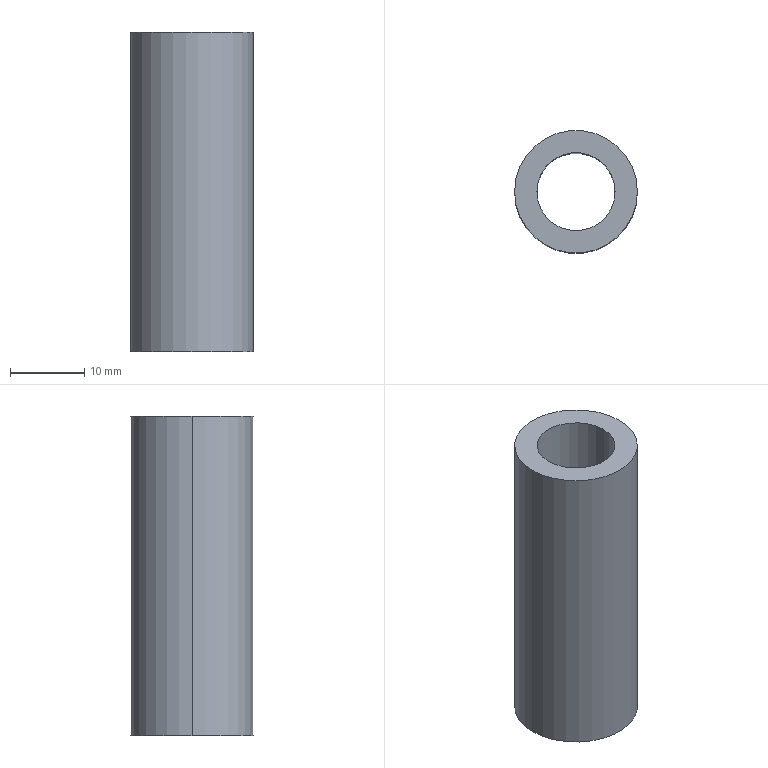Part | SolidWorks | features Extrusion 1, ICE 1 | 1 solid | 6 faces | box 16.5 x 16.5 x 43 mm | volume 5471 mm3 | cylinder 4 | plane 2 | commonest cylinder face diameters 10.5 x2 16.5 x2
STEP:
#1=CARTESIAN_POINT('',(-5.25,0.,0.));
#2=VERTEX_POINT('',#1);
#3=CARTESIAN_POINT('',(5.25,0.,0.));
#4=VERTEX_POINT('',#3);
#5=CARTESIAN_POINT('',(0.,0.,0.));
#6=DIRECTION('',(0.,0.,1.));
#7=DIRECTION('',(1.,0.,0.));
#8=AXIS2_PLACEMENT_3D('',#5,#6,#7);
#9=CIRCLE('',#8,5.25);
#10=EDGE_CURVE('',#2,#4,#9,.T.);
#11=ORIENTED_EDGE('',*,*,#10,.F.);
#12=CARTESIAN_POINT('',(-5.25,0.,43.));
#13=VERTEX_POINT('',#12);
#14=CARTESIAN_POINT('',(-5.25,0.,-57.));
#15=DIRECTION('',(0.,0.,1.));
#16=VECTOR('',#15,1000.);
#17=LINE('',#14,#16);
#18=EDGE_CURVE('',#2,#13,#17,.T.);
#19=ORIENTED_EDGE('',*,*,#18,.T.);
#20=CARTESIAN_POINT('',(5.25,0.,43.));
#21=VERTEX_POINT('',#20);
#22=CARTESIAN_POINT('',(0.,0.,43.));
#23=DIRECTION('',(0.,0.,1.));
#24=DIRECTION('',(1.,0.,0.));
#25=AXIS2_PLACEMENT_3D('',#22,#23,#24);
#26=CIRCLE('',#25,5.25);
#27=EDGE_CURVE('',#13,#21,#26,.T.);
#28=ORIENTED_EDGE('',*,*,#27,.T.);
#29=CARTESIAN_POINT('',(5.25,0.,-57.));
#30=DIRECTION('',(0.,0.,1.));
#31=VECTOR('',#30,1000.);
#32=LINE('',#29,#31);
#33=EDGE_CURVE('',#4,#21,#32,.T.);
#34=ORIENTED_EDGE('',*,*,#33,.F.);
#35=EDGE_LOOP('',(#11,#19,#28,#34));
#36=FACE_OUTER_BOUND('',#35,.T.);
#37=CARTESIAN_POINT('',(0.,0.,-57.));
#38=DIRECTION('',(0.,0.,1.));
#39=DIRECTION('',(1.,0.,0.));
#40=AXIS2_PLACEMENT_3D('',#37,#38,#39);
#41=CYLINDRICAL_SURFACE('',#40,5.25);
#42=ADVANCED_FACE('',(#36),#41,.F.);
#43=CARTESIAN_POINT('',(8.25,0.,43.));
#44=VERTEX_POINT('',#43);
#45=CARTESIAN_POINT('',(-8.25,0.,43.));
#46=VERTEX_POINT('',#45);
#47=CARTESIAN_POINT('',(0.,0.,43.));
#48=DIRECTION('',(0.,0.,1.));
#49=DIRECTION('',(1.,0.,0.));
#50=AXIS2_PLACEMENT_3D('',#47,#48,#49);
#51=CIRCLE('',#50,8.25);
#52=EDGE_CURVE('',#44,#46,#51,.T.);
#53=ORIENTED_EDGE('',*,*,#52,.F.);
#54=CARTESIAN_POINT('',(8.25,0.,0.));
#55=VERTEX_POINT('',#54);
#56=CARTESIAN_POINT('',(8.25,0.,43.));
#57=DIRECTION('',(0.,0.,-1.));
#58=VECTOR('',#57,1000.);
#59=LINE('',#56,#58);
#60=EDGE_CURVE('',#44,#55,#59,.T.);
#61=ORIENTED_EDGE('',*,*,#60,.T.);
#62=CARTESIAN_POINT('',(-8.25,0.,0.));
#63=VERTEX_POINT('',#62);
#64=CARTESIAN_POINT('',(0.,0.,0.));
#65=DIRECTION('',(0.,0.,1.));
#66=DIRECTION('',(1.,0.,0.));
#67=AXIS2_PLACEMENT_3D('',#64,#65,#66);
#68=CIRCLE('',#67,8.25);
#69=EDGE_CURVE('',#55,#63,#68,.T.);
#70=ORIENTED_EDGE('',*,*,#69,.T.);
#71=CARTESIAN_POINT('',(-8.25,0.,43.));
#72=DIRECTION('',(0.,0.,-1.));
#73=VECTOR('',#72,1000.);
#74=LINE('',#71,#73);
#75=EDGE_CURVE('',#46,#63,#74,.T.);
#76=ORIENTED_EDGE('',*,*,#75,.F.);
#77=EDGE_LOOP('',(#53,#61,#70,#76));
#78=FACE_OUTER_BOUND('',#77,.T.);
#79=CARTESIAN_POINT('',(0.,0.,43.));
#80=DIRECTION('',(0.,0.,-1.));
#81=DIRECTION('',(-1.,0.,0.));
#82=AXIS2_PLACEMENT_3D('',#79,#80,#81);
#83=CYLINDRICAL_SURFACE('',#82,8.25);
#84=ADVANCED_FACE('',(#78),#83,.T.);
#85=ORIENTED_EDGE('',*,*,#60,.F.);
#86=CARTESIAN_POINT('',(0.,0.,43.));
#87=DIRECTION('',(0.,0.,1.));
#88=DIRECTION('',(1.,0.,0.));
#89=AXIS2_PLACEMENT_3D('',#86,#87,#88);
#90=CIRCLE('',#89,8.25);
#91=EDGE_CURVE('',#46,#44,#90,.T.);
#92=ORIENTED_EDGE('',*,*,#91,.F.);
#93=ORIENTED_EDGE('',*,*,#75,.T.);
#94=CARTESIAN_POINT('',(0.,0.,0.));
#95=DIRECTION('',(0.,0.,1.));
#96=DIRECTION('',(1.,0.,0.));
#97=AXIS2_PLACEMENT_3D('',#94,#95,#96);
#98=CIRCLE('',#97,8.25);
#99=EDGE_CURVE('',#63,#55,#98,.T.);
#100=ORIENTED_EDGE('',*,*,#99,.T.);
#101=EDGE_LOOP('',(#85,#92,#93,#100));
#102=FACE_OUTER_BOUND('',#101,.T.);
#103=CARTESIAN_POINT('',(0.,0.,43.));
#104=DIRECTION('',(0.,0.,-1.));
#105=DIRECTION('',(-1.,0.,0.));
#106=AXIS2_PLACEMENT_3D('',#103,#104,#105);
#107=CYLINDRICAL_SURFACE('',#106,8.25);
#108=ADVANCED_FACE('',(#102),#107,.T.);
#109=CARTESIAN_POINT('',(0.,0.,43.));
#110=DIRECTION('',(0.,0.,1.));
#111=DIRECTION('',(1.,0.,0.));
#112=AXIS2_PLACEMENT_3D('',#109,#110,#111);
#113=CIRCLE('',#112,5.25);
#114=EDGE_CURVE('',#21,#13,#113,.T.);
#115=ORIENTED_EDGE('',*,*,#114,.F.);
#116=ORIENTED_EDGE('',*,*,#27,.F.);
#117=EDGE_LOOP('',(#115,#116));
#118=FACE_BOUND('',#117,.T.);
#119=ORIENTED_EDGE('',*,*,#91,.T.);
#120=ORIENTED_EDGE('',*,*,#52,.T.);
#121=EDGE_LOOP('',(#119,#120));
#122=FACE_OUTER_BOUND('',#121,.T.);
#123=CARTESIAN_POINT('',(0.,0.,43.));
#124=DIRECTION('',(0.,0.,1.));
#125=DIRECTION('',(1.,0.,0.));
#126=AXIS2_PLACEMENT_3D('',#123,#124,#125);
#127=PLANE('',#126);
#128=ADVANCED_FACE('',(#118,#122),#127,.T.);
#129=CARTESIAN_POINT('',(0.,0.,0.));
#130=DIRECTION('',(0.,0.,1.));
#131=DIRECTION('',(1.,0.,0.));
#132=AXIS2_PLACEMENT_3D('',#129,#130,#131);
#133=CIRCLE('',#132,5.25);
#134=EDGE_CURVE('',#4,#2,#133,.T.);
#135=ORIENTED_EDGE('',*,*,#134,.T.);
#136=ORIENTED_EDGE('',*,*,#10,.T.);
#137=EDGE_LOOP('',(#135,#136));
#138=FACE_BOUND('',#137,.T.);
#139=ORIENTED_EDGE('',*,*,#99,.F.);
#140=ORIENTED_EDGE('',*,*,#69,.F.);
#141=EDGE_LOOP('',(#139,#140));
#142=FACE_OUTER_BOUND('',#141,.T.);
#143=CARTESIAN_POINT('',(0.,0.,0.));
#144=DIRECTION('',(0.,0.,1.));
#145=DIRECTION('',(1.,0.,0.));
#146=AXIS2_PLACEMENT_3D('',#143,#144,#145);
#147=PLANE('',#146);
#148=ADVANCED_FACE('',(#138,#142),#147,.F.);
#149=ORIENTED_EDGE('',*,*,#18,.F.);
#150=ORIENTED_EDGE('',*,*,#134,.F.);
#151=ORIENTED_EDGE('',*,*,#33,.T.);
#152=ORIENTED_EDGE('',*,*,#114,.T.);
#153=EDGE_LOOP('',(#149,#150,#151,#152));
#154=FACE_OUTER_BOUND('',#153,.T.);
#155=CARTESIAN_POINT('',(0.,0.,-57.));
#156=DIRECTION('',(0.,0.,1.));
#157=DIRECTION('',(1.,0.,0.));
#158=AXIS2_PLACEMENT_3D('',#155,#156,#157);
#159=CYLINDRICAL_SURFACE('',#158,5.25);
#160=ADVANCED_FACE('',(#154),#159,.F.);
#161=CLOSED_SHELL('',(#42,#84,#108,#128,#148,#160));
#162=MANIFOLD_SOLID_BREP('',#161);
#163=CARTESIAN_POINT('',(0.,0.,0.));
#164=DIRECTION('',(0.,0.,1.));
#165=DIRECTION('',(1.,0.,0.));
#166=AXIS2_PLACEMENT_3D('',#163,#164,#165);
#167=(LENGTH_UNIT()NAMED_UNIT(*)SI_UNIT(.MILLI.,.METRE.));
#168=UNCERTAINTY_MEASURE_WITH_UNIT(LENGTH_MEASURE(0.00001),#167,'','');
#169=(NAMED_UNIT(*)PLANE_ANGLE_UNIT()SI_UNIT($,.RADIAN.));
#170=(NAMED_UNIT(*)SI_UNIT($,.STERADIAN.)SOLID_ANGLE_UNIT());
#171=(GEOMETRIC_REPRESENTATION_CONTEXT(3)GLOBAL_UNCERTAINTY_ASSIGNED_CONTEXT((#168))GLOBAL_UNIT_ASSIGNED_CONTEXT((#167,#169,#170))REPRESENTATION_CONTEXT('',''));
#172=ADVANCED_BREP_SHAPE_REPRESENTATION('',(#162,#166),#171);